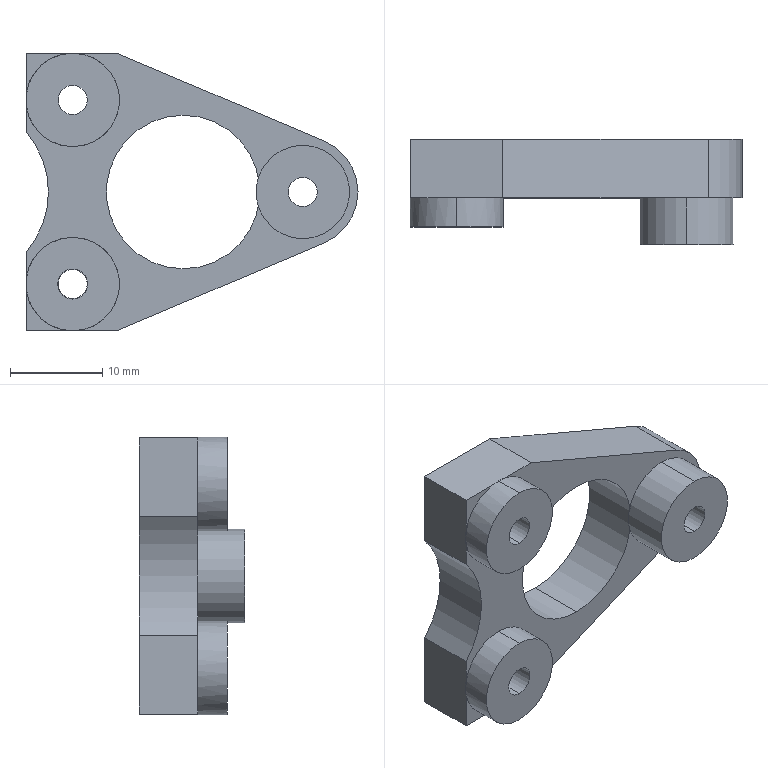Part | SolidWorks | features BaseBody 2 | 2 solids | 39 faces | box 36.08 x 11.43 x 30.16 mm | volume 4168 mm3 | cylinder 20 | plane 19 | commonest cylinder face diameters 3.175 x8 10.16 x6 3.258 x2 16.667 x2 12 x1 20 x1
STEP:
#1=CARTESIAN_POINT('',(-12.,-3.175,-8.371));
#2=VERTEX_POINT('',#1);
#3=CARTESIAN_POINT('',(-12.,-3.175,-11.629));
#4=VERTEX_POINT('',#3);
#5=CARTESIAN_POINT('',(-12.,-3.175,-10.));
#6=DIRECTION('',(0.,-1.,0.));
#7=DIRECTION('',(0.,0.,1.));
#8=AXIS2_PLACEMENT_3D('',#5,#6,#7);
#9=CIRCLE('',#8,1.629);
#10=EDGE_CURVE('',#2,#4,#9,.T.);
#11=ORIENTED_EDGE('',*,*,#10,.T.);
#12=CARTESIAN_POINT('',(-12.,0.,-11.629));
#13=VERTEX_POINT('',#12);
#14=CARTESIAN_POINT('',(-12.,-3.175,-11.629));
#15=DIRECTION('',(0.,1.,0.));
#16=VECTOR('',#15,1000.);
#17=LINE('',#14,#16);
#18=EDGE_CURVE('',#4,#13,#17,.T.);
#19=ORIENTED_EDGE('',*,*,#18,.T.);
#20=CARTESIAN_POINT('',(-12.,0.,-8.371));
#21=VERTEX_POINT('',#20);
#22=CARTESIAN_POINT('',(-12.,0.,-10.));
#23=DIRECTION('',(0.,1.,0.));
#24=DIRECTION('',(0.,0.,1.));
#25=AXIS2_PLACEMENT_3D('',#22,#23,#24);
#26=CIRCLE('',#25,1.629);
#27=EDGE_CURVE('',#13,#21,#26,.T.);
#28=ORIENTED_EDGE('',*,*,#27,.T.);
#29=CARTESIAN_POINT('',(-12.,-3.175,-8.371));
#30=DIRECTION('',(0.,1.,0.));
#31=VECTOR('',#30,1000.);
#32=LINE('',#29,#31);
#33=EDGE_CURVE('',#2,#21,#32,.T.);
#34=ORIENTED_EDGE('',*,*,#33,.F.);
#35=EDGE_LOOP('',(#11,#19,#28,#34));
#36=FACE_OUTER_BOUND('',#35,.T.);
#37=CARTESIAN_POINT('',(-12.,-3.175,-10.));
#38=DIRECTION('',(0.,1.,0.));
#39=DIRECTION('',(0.,0.,1.));
#40=AXIS2_PLACEMENT_3D('',#37,#38,#39);
#41=CYLINDRICAL_SURFACE('',#40,1.629);
#42=ADVANCED_FACE('',(#36),#41,.F.);
#43=CARTESIAN_POINT('',(-12.,6.35,-11.588));
#44=VERTEX_POINT('',#43);
#45=CARTESIAN_POINT('',(-12.,6.35,-8.412));
#46=VERTEX_POINT('',#45);
#47=CARTESIAN_POINT('',(-12.,6.35,-10.));
#48=DIRECTION('',(0.,1.,0.));
#49=DIRECTION('',(0.,0.,-1.));
#50=AXIS2_PLACEMENT_3D('',#47,#48,#49);
#51=CIRCLE('',#50,1.588);
#52=EDGE_CURVE('',#44,#46,#51,.T.);
#53=ORIENTED_EDGE('',*,*,#52,.T.);
#54=CARTESIAN_POINT('',(-12.,0.,-8.412));
#55=VERTEX_POINT('',#54);
#56=CARTESIAN_POINT('',(-12.,6.35,-8.412));
#57=DIRECTION('',(0.,-1.,0.));
#58=VECTOR('',#57,1000.);
#59=LINE('',#56,#58);
#60=EDGE_CURVE('',#46,#55,#59,.T.);
#61=ORIENTED_EDGE('',*,*,#60,.T.);
#62=CARTESIAN_POINT('',(-12.,0.,-11.588));
#63=VERTEX_POINT('',#62);
#64=CARTESIAN_POINT('',(-12.,0.,-10.));
#65=DIRECTION('',(0.,-1.,0.));
#66=DIRECTION('',(0.,0.,-1.));
#67=AXIS2_PLACEMENT_3D('',#64,#65,#66);
#68=CIRCLE('',#67,1.588);
#69=EDGE_CURVE('',#55,#63,#68,.T.);
#70=ORIENTED_EDGE('',*,*,#69,.T.);
#71=CARTESIAN_POINT('',(-12.,6.35,-11.588));
#72=DIRECTION('',(0.,-1.,0.));
#73=VECTOR('',#72,1000.);
#74=LINE('',#71,#73);
#75=EDGE_CURVE('',#44,#63,#74,.T.);
#76=ORIENTED_EDGE('',*,*,#75,.F.);
#77=EDGE_LOOP('',(#53,#61,#70,#76));
#78=FACE_OUTER_BOUND('',#77,.T.);
#79=CARTESIAN_POINT('',(-12.,6.35,-10.));
#80=DIRECTION('',(0.,-1.,0.));
#81=DIRECTION('',(0.,0.,-1.));
#82=AXIS2_PLACEMENT_3D('',#79,#80,#81);
#83=CYLINDRICAL_SURFACE('',#82,1.588);
#84=ADVANCED_FACE('',(#78),#83,.F.);
#85=CARTESIAN_POINT('',(-12.,-3.175,-15.08));
#86=VERTEX_POINT('',#85);
#87=CARTESIAN_POINT('',(-12.,-3.175,-4.92));
#88=VERTEX_POINT('',#87);
#89=CARTESIAN_POINT('',(-12.,-3.175,-10.));
#90=DIRECTION('',(0.,-1.,0.));
#91=DIRECTION('',(0.,0.,1.));
#92=AXIS2_PLACEMENT_3D('',#89,#90,#91);
#93=CIRCLE('',#92,5.08);
#94=EDGE_CURVE('',#86,#88,#93,.T.);
#95=ORIENTED_EDGE('',*,*,#94,.F.);
#96=CARTESIAN_POINT('',(-12.,0.,-15.08));
#97=VERTEX_POINT('',#96);
#98=CARTESIAN_POINT('',(-12.,-3.175,-15.08));
#99=DIRECTION('',(0.,1.,0.));
#100=VECTOR('',#99,1000.);
#101=LINE('',#98,#100);
#102=EDGE_CURVE('',#86,#97,#101,.T.);
#103=ORIENTED_EDGE('',*,*,#102,.T.);
#104=CARTESIAN_POINT('',(-11.102,0.,-15.));
#105=VERTEX_POINT('',#104);
#106=CARTESIAN_POINT('',(-12.,0.,-10.));
#107=DIRECTION('',(0.,-1.,0.));
#108=DIRECTION('',(0.,0.,1.));
#109=AXIS2_PLACEMENT_3D('',#106,#107,#108);
#110=CIRCLE('',#109,5.08);
#111=EDGE_CURVE('',#97,#105,#110,.T.);
#112=ORIENTED_EDGE('',*,*,#111,.T.);
#113=CARTESIAN_POINT('',(-12.,0.,-4.92));
#114=VERTEX_POINT('',#113);
#115=CARTESIAN_POINT('',(-12.,0.,-10.));
#116=DIRECTION('',(0.,1.,0.));
#117=DIRECTION('',(0.,0.,1.));
#118=AXIS2_PLACEMENT_3D('',#115,#116,#117);
#119=CIRCLE('',#118,5.08);
#120=EDGE_CURVE('',#114,#105,#119,.T.);
#121=ORIENTED_EDGE('',*,*,#120,.F.);
#122=CARTESIAN_POINT('',(-12.,-3.175,-4.92));
#123=DIRECTION('',(0.,1.,0.));
#124=VECTOR('',#123,1000.);
#125=LINE('',#122,#124);
#126=EDGE_CURVE('',#88,#114,#125,.T.);
#127=ORIENTED_EDGE('',*,*,#126,.F.);
#128=EDGE_LOOP('',(#95,#103,#112,#121,#127));
#129=FACE_OUTER_BOUND('',#128,.T.);
#130=CARTESIAN_POINT('',(-12.,-3.175,-10.));
#131=DIRECTION('',(0.,1.,0.));
#132=DIRECTION('',(0.,0.,1.));
#133=AXIS2_PLACEMENT_3D('',#130,#131,#132);
#134=CYLINDRICAL_SURFACE('',#133,5.08);
#135=ADVANCED_FACE('',(#129),#134,.T.);
#136=CARTESIAN_POINT('',(13.,6.35,1.587));
#137=VERTEX_POINT('',#136);
#138=CARTESIAN_POINT('',(13.,6.35,-1.587));
#139=VERTEX_POINT('',#138);
#140=CARTESIAN_POINT('',(13.,6.35,0.));
#141=DIRECTION('',(0.,-1.,0.));
#142=DIRECTION('',(0.,0.,-1.));
#143=AXIS2_PLACEMENT_3D('',#140,#141,#142);
#144=CIRCLE('',#143,1.587);
#145=EDGE_CURVE('',#137,#139,#144,.T.);
#146=ORIENTED_EDGE('',*,*,#145,.F.);
#147=CARTESIAN_POINT('',(13.,0.,1.587));
#148=VERTEX_POINT('',#147);
#149=CARTESIAN_POINT('',(13.,6.35,1.587));
#150=DIRECTION('',(0.,-1.,0.));
#151=VECTOR('',#150,1000.);
#152=LINE('',#149,#151);
#153=EDGE_CURVE('',#137,#148,#152,.T.);
#154=ORIENTED_EDGE('',*,*,#153,.T.);
#155=CARTESIAN_POINT('',(13.,0.,-1.587));
#156=VERTEX_POINT('',#155);
#157=CARTESIAN_POINT('',(13.,0.,0.));
#158=DIRECTION('',(0.,-1.,0.));
#159=DIRECTION('',(0.,0.,-1.));
#160=AXIS2_PLACEMENT_3D('',#157,#158,#159);
#161=CIRCLE('',#160,1.587);
#162=EDGE_CURVE('',#148,#156,#161,.T.);
#163=ORIENTED_EDGE('',*,*,#162,.T.);
#164=CARTESIAN_POINT('',(13.,6.35,-1.587));
#165=DIRECTION('',(0.,-1.,0.));
#166=VECTOR('',#165,1000.);
#167=LINE('',#164,#166);
#168=EDGE_CURVE('',#139,#156,#167,.T.);
#169=ORIENTED_EDGE('',*,*,#168,.F.);
#170=EDGE_LOOP('',(#146,#154,#163,#169));
#171=FACE_OUTER_BOUND('',#170,.T.);
#172=CARTESIAN_POINT('',(13.,6.35,0.));
#173=DIRECTION('',(0.,-1.,0.));
#174=DIRECTION('',(0.,0.,-1.));
#175=AXIS2_PLACEMENT_3D('',#172,#173,#174);
#176=CYLINDRICAL_SURFACE('',#175,1.587);
#177=ADVANCED_FACE('',(#171),#176,.F.);
#178=CARTESIAN_POINT('',(-12.,6.35,11.587));
#179=VERTEX_POINT('',#178);
#180=CARTESIAN_POINT('',(-12.,6.35,8.413));
#181=VERTEX_POINT('',#180);
#182=CARTESIAN_POINT('',(-12.,6.35,10.));
#183=DIRECTION('',(0.,-1.,0.));
#184=DIRECTION('',(0.,0.,-1.));
#185=AXIS2_PLACEMENT_3D('',#182,#183,#184);
#186=CIRCLE('',#185,1.587);
#187=EDGE_CURVE('',#179,#181,#186,.T.);
#188=ORIENTED_EDGE('',*,*,#187,.F.);
#189=CARTESIAN_POINT('',(-12.,-3.175,11.587));
#190=VERTEX_POINT('',#189);
#191=CARTESIAN_POINT('',(-12.,6.35,11.587));
#192=DIRECTION('',(0.,-1.,0.));
#193=VECTOR('',#192,1000.);
#194=LINE('',#191,#193);
#195=EDGE_CURVE('',#179,#190,#194,.T.);
#196=ORIENTED_EDGE('',*,*,#195,.T.);
#197=CARTESIAN_POINT('',(-12.,-3.175,8.413));
#198=VERTEX_POINT('',#197);
#199=CARTESIAN_POINT('',(-12.,-3.175,10.));
#200=DIRECTION('',(0.,-1.,0.));
#201=DIRECTION('',(0.,0.,-1.));
#202=AXIS2_PLACEMENT_3D('',#199,#200,#201);
#203=CIRCLE('',#202,1.587);
#204=EDGE_CURVE('',#190,#198,#203,.T.);
#205=ORIENTED_EDGE('',*,*,#204,.T.);
#206=CARTESIAN_POINT('',(-12.,6.35,8.413));
#207=DIRECTION('',(0.,-1.,0.));
#208=VECTOR('',#207,1000.);
#209=LINE('',#206,#208);
#210=EDGE_CURVE('',#181,#198,#209,.T.);
#211=ORIENTED_EDGE('',*,*,#210,.F.);
#212=EDGE_LOOP('',(#188,#196,#205,#211));
#213=FACE_OUTER_BOUND('',#212,.T.);
#214=CARTESIAN_POINT('',(-12.,6.35,10.));
#215=DIRECTION('',(0.,-1.,0.));
#216=DIRECTION('',(0.,0.,-1.));
#217=AXIS2_PLACEMENT_3D('',#214,#215,#216);
#218=CYLINDRICAL_SURFACE('',#217,1.587);
#219=ADVANCED_FACE('',(#213),#218,.F.);
#220=CARTESIAN_POINT('',(0.,6.35,8.334));
#221=VERTEX_POINT('',#220);
#222=CARTESIAN_POINT('',(0.,6.35,-8.334));
#223=VERTEX_POINT('',#222);
#224=CARTESIAN_POINT('',(0.,6.35,0.));
#225=DIRECTION('',(0.,-1.,0.));
#226=DIRECTION('',(0.,0.,-1.));
#227=AXIS2_PLACEMENT_3D('',#224,#225,#226);
#228=CIRCLE('',#227,8.334);
#229=EDGE_CURVE('',#221,#223,#228,.T.);
#230=ORIENTED_EDGE('',*,*,#229,.F.);
#231=CARTESIAN_POINT('',(0.,0.,8.334));
#232=VERTEX_POINT('',#231);
#233=CARTESIAN_POINT('',(0.,6.35,8.334));
#234=DIRECTION('',(0.,-1.,0.));
#235=VECTOR('',#234,1000.);
#236=LINE('',#233,#235);
#237=EDGE_CURVE('',#221,#232,#236,.T.);
#238=ORIENTED_EDGE('',*,*,#237,.T.);
#239=CARTESIAN_POINT('',(0.,0.,-8.334));
#240=VERTEX_POINT('',#239);
#241=CARTESIAN_POINT('',(0.,0.,0.));
#242=DIRECTION('',(0.,-1.,0.));
#243=DIRECTION('',(0.,0.,-1.));
#244=AXIS2_PLACEMENT_3D('',#241,#242,#243);
#245=CIRCLE('',#244,8.334);
#246=EDGE_CURVE('',#232,#240,#245,.T.);
#247=ORIENTED_EDGE('',*,*,#246,.T.);
#248=CARTESIAN_POINT('',(0.,6.35,-8.334));
#249=DIRECTION('',(0.,-1.,0.));
#250=VECTOR('',#249,1000.);
#251=LINE('',#248,#250);
#252=EDGE_CURVE('',#223,#240,#251,.T.);
#253=ORIENTED_EDGE('',*,*,#252,.F.);
#254=EDGE_LOOP('',(#230,#238,#247,#253));
#255=FACE_OUTER_BOUND('',#254,.T.);
#256=CARTESIAN_POINT('',(0.,6.35,0.));
#257=DIRECTION('',(0.,-1.,0.));
#258=DIRECTION('',(0.,0.,-1.));
#259=AXIS2_PLACEMENT_3D('',#256,#257,#258);
#260=CYLINDRICAL_SURFACE('',#259,8.334);
#261=ADVANCED_FACE('',(#255),#260,.F.);
#262=CARTESIAN_POINT('',(-12.,-3.175,4.92));
#263=VERTEX_POINT('',#262);
#264=CARTESIAN_POINT('',(-12.,-3.175,15.08));
#265=VERTEX_POINT('',#264);
#266=CARTESIAN_POINT('',(-12.,-3.175,10.));
#267=DIRECTION('',(0.,-1.,0.));
#268=DIRECTION('',(0.,0.,1.));
#269=AXIS2_PLACEMENT_3D('',#266,#267,#268);
#270=CIRCLE('',#269,5.08);
#271=EDGE_CURVE('',#263,#265,#270,.T.);
#272=ORIENTED_EDGE('',*,*,#271,.F.);
#273=CARTESIAN_POINT('',(-12.,0.,4.92));
#274=VERTEX_POINT('',#273);
#275=CARTESIAN_POINT('',(-12.,-3.175,4.92));
#276=DIRECTION('',(0.,1.,0.));
#277=VECTOR('',#276,1000.);
#278=LINE('',#275,#277);
#279=EDGE_CURVE('',#263,#274,#278,.T.);
#280=ORIENTED_EDGE('',*,*,#279,.T.);
#281=CARTESIAN_POINT('',(-11.102,0.,15.));
#282=VERTEX_POINT('',#281);
#283=CARTESIAN_POINT('',(-12.,0.,10.));
#284=DIRECTION('',(0.,-1.,0.));
#285=DIRECTION('',(0.,0.,1.));
#286=AXIS2_PLACEMENT_3D('',#283,#284,#285);
#287=CIRCLE('',#286,5.08);
#288=EDGE_CURVE('',#274,#282,#287,.T.);
#289=ORIENTED_EDGE('',*,*,#288,.T.);
#290=CARTESIAN_POINT('',(-12.,0.,15.08));
#291=VERTEX_POINT('',#290);
#292=CARTESIAN_POINT('',(-12.,0.,10.));
#293=DIRECTION('',(0.,1.,0.));
#294=DIRECTION('',(0.,0.,1.));
#295=AXIS2_PLACEMENT_3D('',#292,#293,#294);
#296=CIRCLE('',#295,5.08);
#297=EDGE_CURVE('',#291,#282,#296,.T.);
#298=ORIENTED_EDGE('',*,*,#297,.F.);
#299=CARTESIAN_POINT('',(-12.,-3.175,15.08));
#300=DIRECTION('',(0.,1.,0.));
#301=VECTOR('',#300,1000.);
#302=LINE('',#299,#301);
#303=EDGE_CURVE('',#265,#291,#302,.T.);
#304=ORIENTED_EDGE('',*,*,#303,.F.);
#305=EDGE_LOOP('',(#272,#280,#289,#298,#304));
#306=FACE_OUTER_BOUND('',#305,.T.);
#307=CARTESIAN_POINT('',(-12.,-3.175,10.));
#308=DIRECTION('',(0.,1.,0.));
#309=DIRECTION('',(0.,0.,1.));
#310=AXIS2_PLACEMENT_3D('',#307,#308,#309);
#311=CYLINDRICAL_SURFACE('',#310,5.08);
#312=ADVANCED_FACE('',(#306),#311,.T.);
#313=ORIENTED_EDGE('',*,*,#18,.F.);
#314=CARTESIAN_POINT('',(-12.,-3.175,-10.));
#315=DIRECTION('',(0.,-1.,0.));
#316=DIRECTION('',(0.,0.,1.));
#317=AXIS2_PLACEMENT_3D('',#314,#315,#316);
#318=CIRCLE('',#317,1.629);
#319=EDGE_CURVE('',#4,#2,#318,.T.);
#320=ORIENTED_EDGE('',*,*,#319,.T.);
#321=ORIENTED_EDGE('',*,*,#33,.T.);
#322=CARTESIAN_POINT('',(-12.,0.,-10.));
#323=DIRECTION('',(0.,1.,0.));
#324=DIRECTION('',(0.,0.,1.));
#325=AXIS2_PLACEMENT_3D('',#322,#323,#324);
#326=CIRCLE('',#325,1.629);
#327=EDGE_CURVE('',#21,#13,#326,.T.);
#328=ORIENTED_EDGE('',*,*,#327,.T.);
#329=EDGE_LOOP('',(#313,#320,#321,#328));
#330=FACE_OUTER_BOUND('',#329,.T.);
#331=CARTESIAN_POINT('',(-12.,-3.175,-10.));
#332=DIRECTION('',(0.,1.,0.));
#333=DIRECTION('',(0.,0.,1.));
#334=AXIS2_PLACEMENT_3D('',#331,#332,#333);
#335=CYLINDRICAL_SURFACE('',#334,1.629);
#336=ADVANCED_FACE('',(#330),#335,.F.);
#337=CARTESIAN_POINT('',(-12.,0.,-10.));
#338=DIRECTION('',(0.,-1.,0.));
#339=DIRECTION('',(0.,0.,-1.));
#340=AXIS2_PLACEMENT_3D('',#337,#338,#339);
#341=CIRCLE('',#340,1.588);
#342=EDGE_CURVE('',#63,#55,#341,.T.);
#343=ORIENTED_EDGE('',*,*,#342,.F.);
#344=ORIENTED_EDGE('',*,*,#69,.F.);
#345=EDGE_LOOP('',(#343,#344));
#346=FACE_BOUND('',#345,.T.);
#347=ORIENTED_EDGE('',*,*,#327,.F.);
#348=ORIENTED_EDGE('',*,*,#27,.F.);
#349=EDGE_LOOP('',(#347,#348));
#350=FACE_OUTER_BOUND('',#349,.T.);
#351=CARTESIAN_POINT('',(-13.649,0.,-11.649));
#352=DIRECTION('',(0.,1.,0.));
#353=DIRECTION('',(0.,0.,1.));
#354=AXIS2_PLACEMENT_3D('',#351,#352,#353);
#355=PLANE('',#354);
#356=ADVANCED_FACE('',(#346,#350),#355,.F.);
#357=ORIENTED_EDGE('',*,*,#10,.F.);
#358=ORIENTED_EDGE('',*,*,#319,.F.);
#359=EDGE_LOOP('',(#357,#358));
#360=FACE_BOUND('',#359,.T.);
#361=CARTESIAN_POINT('',(-12.,-3.175,-10.));
#362=DIRECTION('',(0.,-1.,0.));
#363=DIRECTION('',(0.,0.,1.));
#364=AXIS2_PLACEMENT_3D('',#361,#362,#363);
#365=CIRCLE('',#364,5.08);
#366=EDGE_CURVE('',#88,#86,#365,.T.);
#367=ORIENTED_EDGE('',*,*,#366,.T.);
#368=ORIENTED_EDGE('',*,*,#94,.T.);
#369=EDGE_LOOP('',(#367,#368));
#370=FACE_OUTER_BOUND('',#369,.T.);
#371=CARTESIAN_POINT('',(-17.141,-3.175,-4.859));
#372=DIRECTION('',(0.,-1.,0.));
#373=DIRECTION('',(0.,0.,-1.));
#374=AXIS2_PLACEMENT_3D('',#371,#372,#373);
#375=PLANE('',#374);
#376=ADVANCED_FACE('',(#360,#370),#375,.T.);
#377=ORIENTED_EDGE('',*,*,#60,.F.);
#378=CARTESIAN_POINT('',(-12.,6.35,-10.));
#379=DIRECTION('',(0.,1.,0.));
#380=DIRECTION('',(0.,0.,-1.));
#381=AXIS2_PLACEMENT_3D('',#378,#379,#380);
#382=CIRCLE('',#381,1.588);
#383=EDGE_CURVE('',#46,#44,#382,.T.);
#384=ORIENTED_EDGE('',*,*,#383,.T.);
#385=ORIENTED_EDGE('',*,*,#75,.T.);
#386=ORIENTED_EDGE('',*,*,#342,.T.);
#387=EDGE_LOOP('',(#377,#384,#385,#386));
#388=FACE_OUTER_BOUND('',#387,.T.);
#389=CARTESIAN_POINT('',(-12.,6.35,-10.));
#390=DIRECTION('',(0.,-1.,0.));
#391=DIRECTION('',(0.,0.,-1.));
#392=AXIS2_PLACEMENT_3D('',#389,#390,#391);
#393=CYLINDRICAL_SURFACE('',#392,1.588);
#394=ADVANCED_FACE('',(#388),#393,.F.);
#395=ORIENTED_EDGE('',*,*,#102,.F.);
#396=ORIENTED_EDGE('',*,*,#366,.F.);
#397=ORIENTED_EDGE('',*,*,#126,.T.);
#398=CARTESIAN_POINT('',(-17.,0.,-9.102));
#399=VERTEX_POINT('',#398);
#400=CARTESIAN_POINT('',(-12.,0.,-10.));
#401=DIRECTION('',(0.,1.,0.));
#402=DIRECTION('',(0.,0.,1.));
#403=AXIS2_PLACEMENT_3D('',#400,#401,#402);
#404=CIRCLE('',#403,5.08);
#405=EDGE_CURVE('',#399,#114,#404,.T.);
#406=ORIENTED_EDGE('',*,*,#405,.F.);
#407=CARTESIAN_POINT('',(-17.,0.,-10.898));
#408=VERTEX_POINT('',#407);
#409=CARTESIAN_POINT('',(-12.,0.,-10.));
#410=DIRECTION('',(0.,1.,0.));
#411=DIRECTION('',(0.,0.,1.));
#412=AXIS2_PLACEMENT_3D('',#409,#410,#411);
#413=CIRCLE('',#412,5.08);
#414=EDGE_CURVE('',#408,#399,#413,.T.);
#415=ORIENTED_EDGE('',*,*,#414,.F.);
#416=CARTESIAN_POINT('',(-12.898,0.,-15.));
#417=VERTEX_POINT('',#416);
#418=CARTESIAN_POINT('',(-12.,0.,-10.));
#419=DIRECTION('',(0.,1.,0.));
#420=DIRECTION('',(0.,0.,1.));
#421=AXIS2_PLACEMENT_3D('',#418,#419,#420);
#422=CIRCLE('',#421,5.08);
#423=EDGE_CURVE('',#417,#408,#422,.T.);
#424=ORIENTED_EDGE('',*,*,#423,.F.);
#425=CARTESIAN_POINT('',(-12.,0.,-10.));
#426=DIRECTION('',(0.,-1.,0.));
#427=DIRECTION('',(0.,0.,1.));
#428=AXIS2_PLACEMENT_3D('',#425,#426,#427);
#429=CIRCLE('',#428,5.08);
#430=EDGE_CURVE('',#417,#97,#429,.T.);
#431=ORIENTED_EDGE('',*,*,#430,.T.);
#432=EDGE_LOOP('',(#395,#396,#397,#406,#415,#424,#431));
#433=FACE_OUTER_BOUND('',#432,.T.);
#434=CARTESIAN_POINT('',(-12.,-3.175,-10.));
#435=DIRECTION('',(0.,1.,0.));
#436=DIRECTION('',(0.,0.,1.));
#437=AXIS2_PLACEMENT_3D('',#434,#435,#436);
#438=CYLINDRICAL_SURFACE('',#437,5.08);
#439=ADVANCED_FACE('',(#433),#438,.T.);
#440=CARTESIAN_POINT('',(13.,6.35,0.));
#441=DIRECTION('',(0.,-1.,0.));
#442=DIRECTION('',(0.,0.,-1.));
#443=AXIS2_PLACEMENT_3D('',#440,#441,#442);
#444=CIRCLE('',#443,1.587);
#445=EDGE_CURVE('',#139,#137,#444,.T.);
#446=ORIENTED_EDGE('',*,*,#445,.T.);
#447=ORIENTED_EDGE('',*,*,#145,.T.);
#448=EDGE_LOOP('',(#446,#447));
#449=FACE_BOUND('',#448,.T.);
#450=CARTESIAN_POINT('',(-12.,6.35,10.));
#451=DIRECTION('',(0.,-1.,0.));
#452=DIRECTION('',(0.,0.,-1.));
#453=AXIS2_PLACEMENT_3D('',#450,#451,#452);
#454=CIRCLE('',#453,1.587);
#455=EDGE_CURVE('',#181,#179,#454,.T.);
#456=ORIENTED_EDGE('',*,*,#455,.T.);
#457=ORIENTED_EDGE('',*,*,#187,.T.);
#458=EDGE_LOOP('',(#456,#457));
#459=FACE_BOUND('',#458,.T.);
#460=ORIENTED_EDGE('',*,*,#52,.F.);
#461=ORIENTED_EDGE('',*,*,#383,.F.);
#462=EDGE_LOOP('',(#460,#461));
#463=FACE_BOUND('',#462,.T.);
#464=CARTESIAN_POINT('',(0.,6.35,0.));
#465=DIRECTION('',(0.,-1.,0.));
#466=DIRECTION('',(0.,0.,-1.));
#467=AXIS2_PLACEMENT_3D('',#464,#465,#466);
#468=CIRCLE('',#467,8.334);
#469=EDGE_CURVE('',#223,#221,#468,.T.);
#470=ORIENTED_EDGE('',*,*,#469,.T.);
#471=ORIENTED_EDGE('',*,*,#229,.T.);
#472=EDGE_LOOP('',(#470,#471));
#473=FACE_BOUND('',#472,.T.);
#474=CARTESIAN_POINT('',(-17.,6.35,-6.455));
#475=VERTEX_POINT('',#474);
#476=CARTESIAN_POINT('',(-17.,6.35,6.455));
#477=VERTEX_POINT('',#476);
#478=CARTESIAN_POINT('',(-24.638,6.35,0.));
#479=DIRECTION('',(0.,-1.,0.));
#480=DIRECTION('',(0.,0.,-1.));
#481=AXIS2_PLACEMENT_3D('',#478,#479,#480);
#482=CIRCLE('',#481,10.);
#483=EDGE_CURVE('',#475,#477,#482,.T.);
#484=ORIENTED_EDGE('',*,*,#483,.T.);
#485=CARTESIAN_POINT('',(-17.,6.35,15.));
#486=VERTEX_POINT('',#485);
#487=CARTESIAN_POINT('',(-17.,6.35,0.));
#488=DIRECTION('',(0.,0.,1.));
#489=VECTOR('',#488,1000.);
#490=LINE('',#487,#489);
#491=EDGE_CURVE('',#477,#486,#490,.T.);
#492=ORIENTED_EDGE('',*,*,#491,.T.);
#493=CARTESIAN_POINT('',(-7.,6.35,15.));
#494=VERTEX_POINT('',#493);
#495=CARTESIAN_POINT('',(1.108,6.35,15.));
#496=DIRECTION('',(1.,0.,0.));
#497=VECTOR('',#496,1000.);
#498=LINE('',#495,#497);
#499=EDGE_CURVE('',#486,#494,#498,.T.);
#500=ORIENTED_EDGE('',*,*,#499,.T.);
#501=CARTESIAN_POINT('',(15.343,6.35,5.524));
#502=VERTEX_POINT('',#501);
#503=CARTESIAN_POINT('',(-7.,6.35,15.));
#504=DIRECTION('',(0.9206,0.,-0.3905));
#505=VECTOR('',#504,1000.);
#506=LINE('',#503,#505);
#507=EDGE_CURVE('',#494,#502,#506,.T.);
#508=ORIENTED_EDGE('',*,*,#507,.T.);
#509=CARTESIAN_POINT('',(15.343,6.35,-5.524));
#510=VERTEX_POINT('',#509);
#511=CARTESIAN_POINT('',(13.,6.35,0.));
#512=DIRECTION('',(0.,1.,0.));
#513=DIRECTION('',(0.,0.,-1.));
#514=AXIS2_PLACEMENT_3D('',#511,#512,#513);
#515=CIRCLE('',#514,6.);
#516=EDGE_CURVE('',#502,#510,#515,.T.);
#517=ORIENTED_EDGE('',*,*,#516,.T.);
#518=CARTESIAN_POINT('',(-7.,6.35,-15.));
#519=VERTEX_POINT('',#518);
#520=CARTESIAN_POINT('',(15.343,6.35,-5.524));
#521=DIRECTION('',(-0.9206,0.,-0.3905));
#522=VECTOR('',#521,1000.);
#523=LINE('',#520,#522);
#524=EDGE_CURVE('',#510,#519,#523,.T.);
#525=ORIENTED_EDGE('',*,*,#524,.T.);
#526=CARTESIAN_POINT('',(-17.,6.35,-15.));
#527=VERTEX_POINT('',#526);
#528=CARTESIAN_POINT('',(1.108,6.35,-15.));
#529=DIRECTION('',(-1.,0.,0.));
#530=VECTOR('',#529,1000.);
#531=LINE('',#528,#530);
#532=EDGE_CURVE('',#519,#527,#531,.T.);
#533=ORIENTED_EDGE('',*,*,#532,.T.);
#534=CARTESIAN_POINT('',(-17.,6.35,0.));
#535=DIRECTION('',(0.,0.,1.));
#536=VECTOR('',#535,1000.);
#537=LINE('',#534,#536);
#538=EDGE_CURVE('',#527,#475,#537,.T.);
#539=ORIENTED_EDGE('',*,*,#538,.T.);
#540=EDGE_LOOP('',(#484,#492,#500,#508,#517,#525,#533,#539));
#541=FACE_OUTER_BOUND('',#540,.T.);
#542=CARTESIAN_POINT('',(-17.,6.35,-15.));
#543=DIRECTION('',(0.,1.,0.));
#544=DIRECTION('',(0.,0.,1.));
#545=AXIS2_PLACEMENT_3D('',#542,#543,#544);
#546=PLANE('',#545);
#547=ADVANCED_FACE('',(#449,#459,#463,#473,#541),#546,.T.);
#548=CARTESIAN_POINT('',(0.,0.,0.));
#549=DIRECTION('',(0.,-1.,0.));
#550=DIRECTION('',(0.,0.,-1.));
#551=AXIS2_PLACEMENT_3D('',#548,#549,#550);
#552=CIRCLE('',#551,8.334);
#553=EDGE_CURVE('',#240,#232,#552,.T.);
#554=ORIENTED_EDGE('',*,*,#553,.F.);
#555=ORIENTED_EDGE('',*,*,#246,.F.);
#556=EDGE_LOOP('',(#554,#555));
#557=FACE_BOUND('',#556,.T.);
#558=CARTESIAN_POINT('',(13.,0.,0.));
#559=DIRECTION('',(0.,-1.,0.));
#560=DIRECTION('',(0.,0.,-1.));
#561=AXIS2_PLACEMENT_3D('',#558,#559,#560);
#562=CIRCLE('',#561,1.587);
#563=EDGE_CURVE('',#156,#148,#562,.T.);
#564=ORIENTED_EDGE('',*,*,#563,.F.);
#565=ORIENTED_EDGE('',*,*,#162,.F.);
#566=EDGE_LOOP('',(#564,#565));
#567=FACE_BOUND('',#566,.T.);
#568=CARTESIAN_POINT('',(-7.,0.,-15.));
#569=VERTEX_POINT('',#568);
#570=CARTESIAN_POINT('',(1.108,0.,-15.));
#571=DIRECTION('',(-1.,0.,0.));
#572=VECTOR('',#571,1000.);
#573=LINE('',#570,#572);
#574=EDGE_CURVE('',#569,#105,#573,.T.);
#575=ORIENTED_EDGE('',*,*,#574,.F.);
#576=CARTESIAN_POINT('',(15.343,0.,-5.524));
#577=VERTEX_POINT('',#576);
#578=CARTESIAN_POINT('',(-7.,0.,-15.));
#579=DIRECTION('',(-0.9206,0.,-0.3905));
#580=VECTOR('',#579,1000.);
#581=LINE('',#578,#580);
#582=EDGE_CURVE('',#577,#569,#581,.T.);
#583=ORIENTED_EDGE('',*,*,#582,.F.);
#584=CARTESIAN_POINT('',(15.343,0.,5.524));
#585=VERTEX_POINT('',#584);
#586=CARTESIAN_POINT('',(13.,0.,0.));
#587=DIRECTION('',(0.,1.,0.));
#588=DIRECTION('',(0.,0.,-1.));
#589=AXIS2_PLACEMENT_3D('',#586,#587,#588);
#590=CIRCLE('',#589,6.);
#591=EDGE_CURVE('',#585,#577,#590,.T.);
#592=ORIENTED_EDGE('',*,*,#591,.F.);
#593=CARTESIAN_POINT('',(-7.,0.,15.));
#594=VERTEX_POINT('',#593);
#595=CARTESIAN_POINT('',(15.343,0.,5.524));
#596=DIRECTION('',(0.9206,0.,-0.3905));
#597=VECTOR('',#596,1000.);
#598=LINE('',#595,#597);
#599=EDGE_CURVE('',#594,#585,#598,.T.);
#600=ORIENTED_EDGE('',*,*,#599,.F.);
#601=CARTESIAN_POINT('',(1.108,0.,15.));
#602=DIRECTION('',(1.,0.,0.));
#603=VECTOR('',#602,1000.);
#604=LINE('',#601,#603);
#605=EDGE_CURVE('',#282,#594,#604,.T.);
#606=ORIENTED_EDGE('',*,*,#605,.F.);
#607=ORIENTED_EDGE('',*,*,#288,.F.);
#608=CARTESIAN_POINT('',(-17.,0.,9.102));
#609=VERTEX_POINT('',#608);
#610=CARTESIAN_POINT('',(-12.,0.,10.));
#611=DIRECTION('',(0.,-1.,0.));
#612=DIRECTION('',(0.,0.,1.));
#613=AXIS2_PLACEMENT_3D('',#610,#611,#612);
#614=CIRCLE('',#613,5.08);
#615=EDGE_CURVE('',#609,#274,#614,.T.);
#616=ORIENTED_EDGE('',*,*,#615,.F.);
#617=CARTESIAN_POINT('',(-17.,0.,6.455));
#618=VERTEX_POINT('',#617);
#619=CARTESIAN_POINT('',(-17.,0.,0.));
#620=DIRECTION('',(0.,0.,1.));
#621=VECTOR('',#620,1000.);
#622=LINE('',#619,#621);
#623=EDGE_CURVE('',#618,#609,#622,.T.);
#624=ORIENTED_EDGE('',*,*,#623,.F.);
#625=CARTESIAN_POINT('',(-17.,0.,-6.455));
#626=VERTEX_POINT('',#625);
#627=CARTESIAN_POINT('',(-24.638,0.,0.));
#628=DIRECTION('',(0.,-1.,0.));
#629=DIRECTION('',(0.,0.,-1.));
#630=AXIS2_PLACEMENT_3D('',#627,#628,#629);
#631=CIRCLE('',#630,10.);
#632=EDGE_CURVE('',#626,#618,#631,.T.);
#633=ORIENTED_EDGE('',*,*,#632,.F.);
#634=CARTESIAN_POINT('',(-17.,0.,0.));
#635=DIRECTION('',(0.,0.,1.));
#636=VECTOR('',#635,1000.);
#637=LINE('',#634,#636);
#638=EDGE_CURVE('',#399,#626,#637,.T.);
#639=ORIENTED_EDGE('',*,*,#638,.F.);
#640=ORIENTED_EDGE('',*,*,#405,.T.);
#641=ORIENTED_EDGE('',*,*,#120,.T.);
#642=EDGE_LOOP('',(#575,#583,#592,#600,#606,#607,#616,#624,#633,#639,#640,#641));
#643=FACE_OUTER_BOUND('',#642,.T.);
#644=CARTESIAN_POINT('',(-17.,0.,-15.));
#645=DIRECTION('',(0.,1.,0.));
#646=DIRECTION('',(0.,0.,1.));
#647=AXIS2_PLACEMENT_3D('',#644,#645,#646);
#648=PLANE('',#647);
#649=ADVANCED_FACE('',(#557,#567,#643),#648,.F.);
#650=CARTESIAN_POINT('',(-17.,0.,-10.));
#651=DIRECTION('',(0.,0.,1.));
#652=VECTOR('',#651,1000.);
#653=LINE('',#650,#652);
#654=EDGE_CURVE('',#408,#399,#653,.T.);
#655=ORIENTED_EDGE('',*,*,#654,.F.);
#656=ORIENTED_EDGE('',*,*,#414,.T.);
#657=EDGE_LOOP('',(#655,#656));
#658=FACE_OUTER_BOUND('',#657,.T.);
#659=CARTESIAN_POINT('',(-17.08,0.,-9.091));
#660=DIRECTION('',(0.,-1.,0.));
#661=DIRECTION('',(0.,0.,-1.));
#662=AXIS2_PLACEMENT_3D('',#659,#660,#661);
#663=PLANE('',#662);
#664=ADVANCED_FACE('',(#658),#663,.F.);
#665=CARTESIAN_POINT('',(-17.,0.,-15.));
#666=VERTEX_POINT('',#665);
#667=CARTESIAN_POINT('',(-17.,0.,-12.937));
#668=DIRECTION('',(0.,0.,1.));
#669=VECTOR('',#668,1000.);
#670=LINE('',#667,#669);
#671=EDGE_CURVE('',#666,#408,#670,.T.);
#672=ORIENTED_EDGE('',*,*,#671,.F.);
#673=CARTESIAN_POINT('',(-14.937,0.,-15.));
#674=DIRECTION('',(-1.,0.,0.));
#675=VECTOR('',#674,1000.);
#676=LINE('',#673,#675);
#677=EDGE_CURVE('',#417,#666,#676,.T.);
#678=ORIENTED_EDGE('',*,*,#677,.F.);
#679=ORIENTED_EDGE('',*,*,#423,.T.);
#680=EDGE_LOOP('',(#672,#678,#679));
#681=FACE_OUTER_BOUND('',#680,.T.);
#682=CARTESIAN_POINT('',(-17.,0.,-15.));
#683=DIRECTION('',(0.,1.,0.));
#684=DIRECTION('',(0.,0.,1.));
#685=AXIS2_PLACEMENT_3D('',#682,#683,#684);
#686=PLANE('',#685);
#687=ADVANCED_FACE('',(#681),#686,.F.);
#688=ORIENTED_EDGE('',*,*,#153,.F.);
#689=ORIENTED_EDGE('',*,*,#445,.F.);
#690=ORIENTED_EDGE('',*,*,#168,.T.);
#691=ORIENTED_EDGE('',*,*,#563,.T.);
#692=EDGE_LOOP('',(#688,#689,#690,#691));
#693=FACE_OUTER_BOUND('',#692,.T.);
#694=CARTESIAN_POINT('',(13.,6.35,0.));
#695=DIRECTION('',(0.,-1.,0.));
#696=DIRECTION('',(0.,0.,-1.));
#697=AXIS2_PLACEMENT_3D('',#694,#695,#696);
#698=CYLINDRICAL_SURFACE('',#697,1.587);
#699=ADVANCED_FACE('',(#693),#698,.F.);
#700=ORIENTED_EDGE('',*,*,#195,.F.);
#701=ORIENTED_EDGE('',*,*,#455,.F.);
#702=ORIENTED_EDGE('',*,*,#210,.T.);
#703=CARTESIAN_POINT('',(-12.,-3.175,10.));
#704=DIRECTION('',(0.,-1.,0.));
#705=DIRECTION('',(0.,0.,-1.));
#706=AXIS2_PLACEMENT_3D('',#703,#704,#705);
#707=CIRCLE('',#706,1.587);
#708=EDGE_CURVE('',#198,#190,#707,.T.);
#709=ORIENTED_EDGE('',*,*,#708,.T.);
#710=EDGE_LOOP('',(#700,#701,#702,#709));
#711=FACE_OUTER_BOUND('',#710,.T.);
#712=CARTESIAN_POINT('',(-12.,6.35,10.));
#713=DIRECTION('',(0.,-1.,0.));
#714=DIRECTION('',(0.,0.,-1.));
#715=AXIS2_PLACEMENT_3D('',#712,#713,#714);
#716=CYLINDRICAL_SURFACE('',#715,1.587);
#717=ADVANCED_FACE('',(#711),#716,.F.);
#718=ORIENTED_EDGE('',*,*,#237,.F.);
#719=ORIENTED_EDGE('',*,*,#469,.F.);
#720=ORIENTED_EDGE('',*,*,#252,.T.);
#721=ORIENTED_EDGE('',*,*,#553,.T.);
#722=EDGE_LOOP('',(#718,#719,#720,#721));
#723=FACE_OUTER_BOUND('',#722,.T.);
#724=CARTESIAN_POINT('',(0.,6.35,0.));
#725=DIRECTION('',(0.,-1.,0.));
#726=DIRECTION('',(0.,0.,-1.));
#727=AXIS2_PLACEMENT_3D('',#724,#725,#726);
#728=CYLINDRICAL_SURFACE('',#727,8.334);
#729=ADVANCED_FACE('',(#723),#728,.F.);
#730=CARTESIAN_POINT('',(-17.,0.,10.898));
#731=VERTEX_POINT('',#730);
#732=CARTESIAN_POINT('',(-17.,0.,10.727));
#733=DIRECTION('',(0.,0.,-1.));
#734=VECTOR('',#733,1000.);
#735=LINE('',#732,#734);
#736=EDGE_CURVE('',#731,#609,#735,.T.);
#737=ORIENTED_EDGE('',*,*,#736,.F.);
#738=CARTESIAN_POINT('',(-17.,0.,15.));
#739=VERTEX_POINT('',#738);
#740=CARTESIAN_POINT('',(-17.,0.,10.727));
#741=DIRECTION('',(0.,0.,-1.));
#742=VECTOR('',#741,1000.);
#743=LINE('',#740,#742);
#744=EDGE_CURVE('',#739,#731,#743,.T.);
#745=ORIENTED_EDGE('',*,*,#744,.F.);
#746=CARTESIAN_POINT('',(-17.,3.175,15.));
#747=DIRECTION('',(0.,-1.,0.));
#748=VECTOR('',#747,1000.);
#749=LINE('',#746,#748);
#750=EDGE_CURVE('',#486,#739,#749,.T.);
#751=ORIENTED_EDGE('',*,*,#750,.F.);
#752=ORIENTED_EDGE('',*,*,#491,.F.);
#753=CARTESIAN_POINT('',(-17.,3.175,6.455));
#754=DIRECTION('',(0.,1.,0.));
#755=VECTOR('',#754,1000.);
#756=LINE('',#753,#755);
#757=EDGE_CURVE('',#618,#477,#756,.T.);
#758=ORIENTED_EDGE('',*,*,#757,.F.);
#759=ORIENTED_EDGE('',*,*,#623,.T.);
#760=EDGE_LOOP('',(#737,#745,#751,#752,#758,#759));
#761=FACE_OUTER_BOUND('',#760,.T.);
#762=CARTESIAN_POINT('',(-17.,0.,15.));
#763=DIRECTION('',(1.,0.,0.));
#764=DIRECTION('',(0.,0.,-1.));
#765=AXIS2_PLACEMENT_3D('',#762,#763,#764);
#766=PLANE('',#765);
#767=ADVANCED_FACE('',(#761),#766,.F.);
#768=ORIENTED_EDGE('',*,*,#483,.F.);
#769=CARTESIAN_POINT('',(-17.,3.175,-6.455));
#770=DIRECTION('',(0.,-1.,0.));
#771=VECTOR('',#770,1000.);
#772=LINE('',#769,#771);
#773=EDGE_CURVE('',#475,#626,#772,.T.);
#774=ORIENTED_EDGE('',*,*,#773,.T.);
#775=ORIENTED_EDGE('',*,*,#632,.T.);
#776=ORIENTED_EDGE('',*,*,#757,.T.);
#777=EDGE_LOOP('',(#768,#774,#775,#776));
#778=FACE_OUTER_BOUND('',#777,.T.);
#779=CARTESIAN_POINT('',(-24.638,6.35,0.));
#780=DIRECTION('',(0.,-1.,0.));
#781=DIRECTION('',(0.,0.,-1.));
#782=AXIS2_PLACEMENT_3D('',#779,#780,#781);
#783=CYLINDRICAL_SURFACE('',#782,10.);
#784=ADVANCED_FACE('',(#778),#783,.F.);
#785=ORIENTED_EDGE('',*,*,#654,.T.);
#786=ORIENTED_EDGE('',*,*,#638,.T.);
#787=ORIENTED_EDGE('',*,*,#773,.F.);
#788=ORIENTED_EDGE('',*,*,#538,.F.);
#789=CARTESIAN_POINT('',(-17.,3.175,-15.));
#790=DIRECTION('',(0.,1.,0.));
#791=VECTOR('',#790,1000.);
#792=LINE('',#789,#791);
#793=EDGE_CURVE('',#666,#527,#792,.T.);
#794=ORIENTED_EDGE('',*,*,#793,.F.);
#795=ORIENTED_EDGE('',*,*,#671,.T.);
#796=EDGE_LOOP('',(#785,#786,#787,#788,#794,#795));
#797=FACE_OUTER_BOUND('',#796,.T.);
#798=CARTESIAN_POINT('',(-17.,0.,-6.455));
#799=DIRECTION('',(1.,0.,0.));
#800=DIRECTION('',(0.,0.,-1.));
#801=AXIS2_PLACEMENT_3D('',#798,#799,#800);
#802=PLANE('',#801);
#803=ADVANCED_FACE('',(#797),#802,.F.);
#804=CARTESIAN_POINT('',(-12.,0.,-15.));
#805=DIRECTION('',(1.,0.,0.));
#806=VECTOR('',#805,1000.);
#807=LINE('',#804,#806);
#808=EDGE_CURVE('',#417,#105,#807,.T.);
#809=ORIENTED_EDGE('',*,*,#808,.F.);
#810=ORIENTED_EDGE('',*,*,#677,.T.);
#811=ORIENTED_EDGE('',*,*,#793,.T.);
#812=ORIENTED_EDGE('',*,*,#532,.F.);
#813=CARTESIAN_POINT('',(-7.,3.175,-15.));
#814=DIRECTION('',(0.,1.,0.));
#815=VECTOR('',#814,1000.);
#816=LINE('',#813,#815);
#817=EDGE_CURVE('',#569,#519,#816,.T.);
#818=ORIENTED_EDGE('',*,*,#817,.F.);
#819=ORIENTED_EDGE('',*,*,#574,.T.);
#820=EDGE_LOOP('',(#809,#810,#811,#812,#818,#819));
#821=FACE_OUTER_BOUND('',#820,.T.);
#822=CARTESIAN_POINT('',(-17.,0.,-15.));
#823=DIRECTION('',(0.,0.,1.));
#824=DIRECTION('',(1.,0.,0.));
#825=AXIS2_PLACEMENT_3D('',#822,#823,#824);
#826=PLANE('',#825);
#827=ADVANCED_FACE('',(#821),#826,.F.);
#828=ORIENTED_EDGE('',*,*,#817,.T.);
#829=ORIENTED_EDGE('',*,*,#524,.F.);
#830=CARTESIAN_POINT('',(15.343,3.175,-5.524));
#831=DIRECTION('',(0.,1.,0.));
#832=VECTOR('',#831,1000.);
#833=LINE('',#830,#832);
#834=EDGE_CURVE('',#577,#510,#833,.T.);
#835=ORIENTED_EDGE('',*,*,#834,.F.);
#836=ORIENTED_EDGE('',*,*,#582,.T.);
#837=EDGE_LOOP('',(#828,#829,#835,#836));
#838=FACE_OUTER_BOUND('',#837,.T.);
#839=CARTESIAN_POINT('',(-7.,0.,-15.));
#840=DIRECTION('',(-0.3905,0.,0.9206));
#841=DIRECTION('',(0.9206,0.,0.3905));
#842=AXIS2_PLACEMENT_3D('',#839,#840,#841);
#843=PLANE('',#842);
#844=ADVANCED_FACE('',(#838),#843,.F.);
#845=ORIENTED_EDGE('',*,*,#834,.T.);
#846=ORIENTED_EDGE('',*,*,#516,.F.);
#847=CARTESIAN_POINT('',(15.343,3.175,5.524));
#848=DIRECTION('',(0.,1.,0.));
#849=VECTOR('',#848,1000.);
#850=LINE('',#847,#849);
#851=EDGE_CURVE('',#585,#502,#850,.T.);
#852=ORIENTED_EDGE('',*,*,#851,.F.);
#853=ORIENTED_EDGE('',*,*,#591,.T.);
#854=EDGE_LOOP('',(#845,#846,#852,#853));
#855=FACE_OUTER_BOUND('',#854,.T.);
#856=CARTESIAN_POINT('',(13.,6.35,0.));
#857=DIRECTION('',(0.,-1.,0.));
#858=DIRECTION('',(0.,0.,-1.));
#859=AXIS2_PLACEMENT_3D('',#856,#857,#858);
#860=CYLINDRICAL_SURFACE('',#859,6.);
#861=ADVANCED_FACE('',(#855),#860,.T.);
#862=ORIENTED_EDGE('',*,*,#851,.T.);
#863=ORIENTED_EDGE('',*,*,#507,.F.);
#864=CARTESIAN_POINT('',(-7.,3.175,15.));
#865=DIRECTION('',(0.,1.,0.));
#866=VECTOR('',#865,1000.);
#867=LINE('',#864,#866);
#868=EDGE_CURVE('',#594,#494,#867,.T.);
#869=ORIENTED_EDGE('',*,*,#868,.F.);
#870=ORIENTED_EDGE('',*,*,#599,.T.);
#871=EDGE_LOOP('',(#862,#863,#869,#870));
#872=FACE_OUTER_BOUND('',#871,.T.);
#873=CARTESIAN_POINT('',(15.343,0.,5.524));
#874=DIRECTION('',(-0.3905,0.,-0.9206));
#875=DIRECTION('',(-0.9206,0.,0.3905));
#876=AXIS2_PLACEMENT_3D('',#873,#874,#875);
#877=PLANE('',#876);
#878=ADVANCED_FACE('',(#872),#877,.F.);
#879=CARTESIAN_POINT('',(-12.898,0.,15.));
#880=VERTEX_POINT('',#879);
#881=CARTESIAN_POINT('',(-12.,0.,15.));
#882=DIRECTION('',(-1.,0.,0.));
#883=VECTOR('',#882,1000.);
#884=LINE('',#881,#883);
#885=EDGE_CURVE('',#282,#880,#884,.T.);
#886=ORIENTED_EDGE('',*,*,#885,.F.);
#887=ORIENTED_EDGE('',*,*,#605,.T.);
#888=ORIENTED_EDGE('',*,*,#868,.T.);
#889=ORIENTED_EDGE('',*,*,#499,.F.);
#890=ORIENTED_EDGE('',*,*,#750,.T.);
#891=CARTESIAN_POINT('',(-12.,0.,15.));
#892=DIRECTION('',(-1.,0.,0.));
#893=VECTOR('',#892,1000.);
#894=LINE('',#891,#893);
#895=EDGE_CURVE('',#880,#739,#894,.T.);
#896=ORIENTED_EDGE('',*,*,#895,.F.);
#897=EDGE_LOOP('',(#886,#887,#888,#889,#890,#896));
#898=FACE_OUTER_BOUND('',#897,.T.);
#899=CARTESIAN_POINT('',(-7.,0.,15.));
#900=DIRECTION('',(0.,0.,-1.));
#901=DIRECTION('',(-1.,0.,0.));
#902=AXIS2_PLACEMENT_3D('',#899,#900,#901);
#903=PLANE('',#902);
#904=ADVANCED_FACE('',(#898),#903,.F.);
#905=ORIENTED_EDGE('',*,*,#279,.F.);
#906=CARTESIAN_POINT('',(-12.,-3.175,10.));
#907=DIRECTION('',(0.,-1.,0.));
#908=DIRECTION('',(0.,0.,1.));
#909=AXIS2_PLACEMENT_3D('',#906,#907,#908);
#910=CIRCLE('',#909,5.08);
#911=EDGE_CURVE('',#265,#263,#910,.T.);
#912=ORIENTED_EDGE('',*,*,#911,.F.);
#913=ORIENTED_EDGE('',*,*,#303,.T.);
#914=CARTESIAN_POINT('',(-12.,0.,10.));
#915=DIRECTION('',(0.,1.,0.));
#916=DIRECTION('',(0.,0.,1.));
#917=AXIS2_PLACEMENT_3D('',#914,#915,#916);
#918=CIRCLE('',#917,5.08);
#919=EDGE_CURVE('',#880,#291,#918,.T.);
#920=ORIENTED_EDGE('',*,*,#919,.F.);
#921=CARTESIAN_POINT('',(-12.,0.,10.));
#922=DIRECTION('',(0.,1.,0.));
#923=DIRECTION('',(0.,0.,1.));
#924=AXIS2_PLACEMENT_3D('',#921,#922,#923);
#925=CIRCLE('',#924,5.08);
#926=EDGE_CURVE('',#731,#880,#925,.T.);
#927=ORIENTED_EDGE('',*,*,#926,.F.);
#928=CARTESIAN_POINT('',(-12.,0.,10.));
#929=DIRECTION('',(0.,1.,0.));
#930=DIRECTION('',(0.,0.,1.));
#931=AXIS2_PLACEMENT_3D('',#928,#929,#930);
#932=CIRCLE('',#931,5.08);
#933=EDGE_CURVE('',#609,#731,#932,.T.);
#934=ORIENTED_EDGE('',*,*,#933,.F.);
#935=ORIENTED_EDGE('',*,*,#615,.T.);
#936=EDGE_LOOP('',(#905,#912,#913,#920,#927,#934,#935));
#937=FACE_OUTER_BOUND('',#936,.T.);
#938=CARTESIAN_POINT('',(-12.,-3.175,10.));
#939=DIRECTION('',(0.,1.,0.));
#940=DIRECTION('',(0.,0.,1.));
#941=AXIS2_PLACEMENT_3D('',#938,#939,#940);
#942=CYLINDRICAL_SURFACE('',#941,5.08);
#943=ADVANCED_FACE('',(#937),#942,.T.);
#944=ORIENTED_EDGE('',*,*,#708,.F.);
#945=ORIENTED_EDGE('',*,*,#204,.F.);
#946=EDGE_LOOP('',(#944,#945));
#947=FACE_BOUND('',#946,.T.);
#948=ORIENTED_EDGE('',*,*,#911,.T.);
#949=ORIENTED_EDGE('',*,*,#271,.T.);
#950=EDGE_LOOP('',(#948,#949));
#951=FACE_OUTER_BOUND('',#950,.T.);
#952=CARTESIAN_POINT('',(-17.141,-3.175,15.141));
#953=DIRECTION('',(0.,-1.,0.));
#954=DIRECTION('',(0.,0.,-1.));
#955=AXIS2_PLACEMENT_3D('',#952,#953,#954);
#956=PLANE('',#955);
#957=ADVANCED_FACE('',(#947,#951),#956,.T.);
#958=ORIENTED_EDGE('',*,*,#933,.T.);
#959=ORIENTED_EDGE('',*,*,#736,.T.);
#960=EDGE_LOOP('',(#958,#959));
#961=FACE_OUTER_BOUND('',#960,.T.);
#962=CARTESIAN_POINT('',(-17.08,0.,10.909));
#963=DIRECTION('',(0.,-1.,0.));
#964=DIRECTION('',(0.,0.,-1.));
#965=AXIS2_PLACEMENT_3D('',#962,#963,#964);
#966=PLANE('',#965);
#967=ADVANCED_FACE('',(#961),#966,.F.);
#968=ORIENTED_EDGE('',*,*,#895,.T.);
#969=ORIENTED_EDGE('',*,*,#744,.T.);
#970=ORIENTED_EDGE('',*,*,#926,.T.);
#971=EDGE_LOOP('',(#968,#969,#970));
#972=FACE_OUTER_BOUND('',#971,.T.);
#973=CARTESIAN_POINT('',(-17.,0.,10.873));
#974=DIRECTION('',(0.,1.,0.));
#975=DIRECTION('',(0.,0.,1.));
#976=AXIS2_PLACEMENT_3D('',#973,#974,#975);
#977=PLANE('',#976);
#978=ADVANCED_FACE('',(#972),#977,.F.);
#979=ORIENTED_EDGE('',*,*,#808,.T.);
#980=ORIENTED_EDGE('',*,*,#111,.F.);
#981=ORIENTED_EDGE('',*,*,#430,.F.);
#982=EDGE_LOOP('',(#979,#980,#981));
#983=FACE_OUTER_BOUND('',#982,.T.);
#984=CARTESIAN_POINT('',(-12.909,0.,-15.));
#985=DIRECTION('',(0.,-1.,0.));
#986=DIRECTION('',(0.,0.,-1.));
#987=AXIS2_PLACEMENT_3D('',#984,#985,#986);
#988=PLANE('',#987);
#989=ADVANCED_FACE('',(#983),#988,.F.);
#990=ORIENTED_EDGE('',*,*,#885,.T.);
#991=ORIENTED_EDGE('',*,*,#919,.T.);
#992=ORIENTED_EDGE('',*,*,#297,.T.);
#993=EDGE_LOOP('',(#990,#991,#992));
#994=FACE_OUTER_BOUND('',#993,.T.);
#995=CARTESIAN_POINT('',(-12.909,0.,15.08));
#996=DIRECTION('',(0.,-1.,0.));
#997=DIRECTION('',(0.,0.,-1.));
#998=AXIS2_PLACEMENT_3D('',#995,#996,#997);
#999=PLANE('',#998);
#1000=ADVANCED_FACE('',(#994),#999,.F.);
#1001=CLOSED_SHELL('',(#42,#84,#135,#177,#219,#261,#312,#336,#356,#376,#394,#439,#547,#649,#664,#687,#699,#717,#729,#767,#784,#803,#827,#844,#861,#878,#904,#943,#957,#967,#978,#989,#1000));
#1002=MANIFOLD_SOLID_BREP('',#1001);
#1003=CARTESIAN_POINT('',(13.,-5.08,1.587));
#1004=VERTEX_POINT('',#1003);
#1005=CARTESIAN_POINT('',(13.,-5.08,-1.587));
#1006=VERTEX_POINT('',#1005);
#1007=CARTESIAN_POINT('',(13.,-5.08,0.));
#1008=DIRECTION('',(0.,-1.,0.));
#1009=DIRECTION('',(0.,0.,1.));
#1010=AXIS2_PLACEMENT_3D('',#1007,#1008,#1009);
#1011=CIRCLE('',#1010,1.587);
#1012=EDGE_CURVE('',#1004,#1006,#1011,.T.);
#1013=ORIENTED_EDGE('',*,*,#1012,.T.);
#1014=CARTESIAN_POINT('',(13.,0.,-1.587));
#1015=VERTEX_POINT('',#1014);
#1016=CARTESIAN_POINT('',(13.,-5.08,-1.587));
#1017=DIRECTION('',(0.,1.,0.));
#1018=VECTOR('',#1017,1000.);
#1019=LINE('',#1016,#1018);
#1020=EDGE_CURVE('',#1006,#1015,#1019,.T.);
#1021=ORIENTED_EDGE('',*,*,#1020,.T.);
#1022=CARTESIAN_POINT('',(13.,0.,1.587));
#1023=VERTEX_POINT('',#1022);
#1024=CARTESIAN_POINT('',(13.,0.,0.));
#1025=DIRECTION('',(0.,1.,0.));
#1026=DIRECTION('',(0.,0.,1.));
#1027=AXIS2_PLACEMENT_3D('',#1024,#1025,#1026);
#1028=CIRCLE('',#1027,1.587);
#1029=EDGE_CURVE('',#1015,#1023,#1028,.T.);
#1030=ORIENTED_EDGE('',*,*,#1029,.T.);
#1031=CARTESIAN_POINT('',(13.,-5.08,1.587));
#1032=DIRECTION('',(0.,1.,0.));
#1033=VECTOR('',#1032,1000.);
#1034=LINE('',#1031,#1033);
#1035=EDGE_CURVE('',#1004,#1023,#1034,.T.);
#1036=ORIENTED_EDGE('',*,*,#1035,.F.);
#1037=EDGE_LOOP('',(#1013,#1021,#1030,#1036));
#1038=FACE_OUTER_BOUND('',#1037,.T.);
#1039=CARTESIAN_POINT('',(13.,-5.08,0.));
#1040=DIRECTION('',(0.,1.,0.));
#1041=DIRECTION('',(0.,0.,1.));
#1042=AXIS2_PLACEMENT_3D('',#1039,#1040,#1041);
#1043=CYLINDRICAL_SURFACE('',#1042,1.587);
#1044=ADVANCED_FACE('',(#1038),#1043,.F.);
#1045=CARTESIAN_POINT('',(13.,-5.08,-5.08));
#1046=VERTEX_POINT('',#1045);
#1047=CARTESIAN_POINT('',(13.,-5.08,5.08));
#1048=VERTEX_POINT('',#1047);
#1049=CARTESIAN_POINT('',(13.,-5.08,0.));
#1050=DIRECTION('',(0.,-1.,0.));
#1051=DIRECTION('',(0.,0.,1.));
#1052=AXIS2_PLACEMENT_3D('',#1049,#1050,#1051);
#1053=CIRCLE('',#1052,5.08);
#1054=EDGE_CURVE('',#1046,#1048,#1053,.T.);
#1055=ORIENTED_EDGE('',*,*,#1054,.F.);
#1056=CARTESIAN_POINT('',(13.,0.,-5.08));
#1057=VERTEX_POINT('',#1056);
#1058=CARTESIAN_POINT('',(13.,-5.08,-5.08));
#1059=DIRECTION('',(0.,1.,0.));
#1060=VECTOR('',#1059,1000.);
#1061=LINE('',#1058,#1060);
#1062=EDGE_CURVE('',#1046,#1057,#1061,.T.);
#1063=ORIENTED_EDGE('',*,*,#1062,.T.);
#1064=CARTESIAN_POINT('',(13.,0.,5.08));
#1065=VERTEX_POINT('',#1064);
#1066=CARTESIAN_POINT('',(13.,0.,0.));
#1067=DIRECTION('',(0.,-1.,0.));
#1068=DIRECTION('',(0.,0.,1.));
#1069=AXIS2_PLACEMENT_3D('',#1066,#1067,#1068);
#1070=CIRCLE('',#1069,5.08);
#1071=EDGE_CURVE('',#1057,#1065,#1070,.T.);
#1072=ORIENTED_EDGE('',*,*,#1071,.T.);
#1073=CARTESIAN_POINT('',(13.,-5.08,5.08));
#1074=DIRECTION('',(0.,1.,0.));
#1075=VECTOR('',#1074,1000.);
#1076=LINE('',#1073,#1075);
#1077=EDGE_CURVE('',#1048,#1065,#1076,.T.);
#1078=ORIENTED_EDGE('',*,*,#1077,.F.);
#1079=EDGE_LOOP('',(#1055,#1063,#1072,#1078));
#1080=FACE_OUTER_BOUND('',#1079,.T.);
#1081=CARTESIAN_POINT('',(13.,-5.08,0.));
#1082=DIRECTION('',(0.,1.,0.));
#1083=DIRECTION('',(0.,0.,1.));
#1084=AXIS2_PLACEMENT_3D('',#1081,#1082,#1083);
#1085=CYLINDRICAL_SURFACE('',#1084,5.08);
#1086=ADVANCED_FACE('',(#1080),#1085,.T.);
#1087=ORIENTED_EDGE('',*,*,#1020,.F.);
#1088=CARTESIAN_POINT('',(13.,-5.08,0.));
#1089=DIRECTION('',(0.,-1.,0.));
#1090=DIRECTION('',(0.,0.,1.));
#1091=AXIS2_PLACEMENT_3D('',#1088,#1089,#1090);
#1092=CIRCLE('',#1091,1.587);
#1093=EDGE_CURVE('',#1006,#1004,#1092,.T.);
#1094=ORIENTED_EDGE('',*,*,#1093,.T.);
#1095=ORIENTED_EDGE('',*,*,#1035,.T.);
#1096=CARTESIAN_POINT('',(13.,0.,0.));
#1097=DIRECTION('',(0.,1.,0.));
#1098=DIRECTION('',(0.,0.,1.));
#1099=AXIS2_PLACEMENT_3D('',#1096,#1097,#1098);
#1100=CIRCLE('',#1099,1.587);
#1101=EDGE_CURVE('',#1023,#1015,#1100,.T.);
#1102=ORIENTED_EDGE('',*,*,#1101,.T.);
#1103=EDGE_LOOP('',(#1087,#1094,#1095,#1102));
#1104=FACE_OUTER_BOUND('',#1103,.T.);
#1105=CARTESIAN_POINT('',(13.,-5.08,0.));
#1106=DIRECTION('',(0.,1.,0.));
#1107=DIRECTION('',(0.,0.,1.));
#1108=AXIS2_PLACEMENT_3D('',#1105,#1106,#1107);
#1109=CYLINDRICAL_SURFACE('',#1108,1.587);
#1110=ADVANCED_FACE('',(#1104),#1109,.F.);
#1111=ORIENTED_EDGE('',*,*,#1101,.F.);
#1112=ORIENTED_EDGE('',*,*,#1029,.F.);
#1113=EDGE_LOOP('',(#1111,#1112));
#1114=FACE_BOUND('',#1113,.T.);
#1115=CARTESIAN_POINT('',(13.,0.,0.));
#1116=DIRECTION('',(0.,-1.,0.));
#1117=DIRECTION('',(0.,0.,1.));
#1118=AXIS2_PLACEMENT_3D('',#1115,#1116,#1117);
#1119=CIRCLE('',#1118,5.08);
#1120=EDGE_CURVE('',#1065,#1057,#1119,.T.);
#1121=ORIENTED_EDGE('',*,*,#1120,.F.);
#1122=ORIENTED_EDGE('',*,*,#1071,.F.);
#1123=EDGE_LOOP('',(#1121,#1122));
#1124=FACE_OUTER_BOUND('',#1123,.T.);
#1125=CARTESIAN_POINT('',(7.859,0.,5.141));
#1126=DIRECTION('',(0.,-1.,0.));
#1127=DIRECTION('',(0.,0.,-1.));
#1128=AXIS2_PLACEMENT_3D('',#1125,#1126,#1127);
#1129=PLANE('',#1128);
#1130=ADVANCED_FACE('',(#1114,#1124),#1129,.F.);
#1131=ORIENTED_EDGE('',*,*,#1012,.F.);
#1132=ORIENTED_EDGE('',*,*,#1093,.F.);
#1133=EDGE_LOOP('',(#1131,#1132));
#1134=FACE_BOUND('',#1133,.T.);
#1135=CARTESIAN_POINT('',(13.,-5.08,0.));
#1136=DIRECTION('',(0.,-1.,0.));
#1137=DIRECTION('',(0.,0.,1.));
#1138=AXIS2_PLACEMENT_3D('',#1135,#1136,#1137);
#1139=CIRCLE('',#1138,5.08);
#1140=EDGE_CURVE('',#1048,#1046,#1139,.T.);
#1141=ORIENTED_EDGE('',*,*,#1140,.T.);
#1142=ORIENTED_EDGE('',*,*,#1054,.T.);
#1143=EDGE_LOOP('',(#1141,#1142));
#1144=FACE_OUTER_BOUND('',#1143,.T.);
#1145=CARTESIAN_POINT('',(7.859,-5.08,5.141));
#1146=DIRECTION('',(0.,-1.,0.));
#1147=DIRECTION('',(0.,0.,-1.));
#1148=AXIS2_PLACEMENT_3D('',#1145,#1146,#1147);
#1149=PLANE('',#1148);
#1150=ADVANCED_FACE('',(#1134,#1144),#1149,.T.);
#1151=ORIENTED_EDGE('',*,*,#1062,.F.);
#1152=ORIENTED_EDGE('',*,*,#1140,.F.);
#1153=ORIENTED_EDGE('',*,*,#1077,.T.);
#1154=ORIENTED_EDGE('',*,*,#1120,.T.);
#1155=EDGE_LOOP('',(#1151,#1152,#1153,#1154));
#1156=FACE_OUTER_BOUND('',#1155,.T.);
#1157=CARTESIAN_POINT('',(13.,-5.08,0.));
#1158=DIRECTION('',(0.,1.,0.));
#1159=DIRECTION('',(0.,0.,1.));
#1160=AXIS2_PLACEMENT_3D('',#1157,#1158,#1159);
#1161=CYLINDRICAL_SURFACE('',#1160,5.08);
#1162=ADVANCED_FACE('',(#1156),#1161,.T.);
#1163=CLOSED_SHELL('',(#1044,#1086,#1110,#1130,#1150,#1162));
#1164=MANIFOLD_SOLID_BREP('',#1163);
#1165=CARTESIAN_POINT('',(0.,0.,0.));
#1166=DIRECTION('',(0.,0.,1.));
#1167=DIRECTION('',(1.,0.,0.));
#1168=AXIS2_PLACEMENT_3D('',#1165,#1166,#1167);
#1169=(LENGTH_UNIT()NAMED_UNIT(*)SI_UNIT(.MILLI.,.METRE.));
#1170=UNCERTAINTY_MEASURE_WITH_UNIT(LENGTH_MEASURE(0.00001),#1169,'','');
#1171=(NAMED_UNIT(*)PLANE_ANGLE_UNIT()SI_UNIT($,.RADIAN.));
#1172=(NAMED_UNIT(*)SI_UNIT($,.STERADIAN.)SOLID_ANGLE_UNIT());
#1173=(GEOMETRIC_REPRESENTATION_CONTEXT(3)GLOBAL_UNCERTAINTY_ASSIGNED_CONTEXT((#1170))GLOBAL_UNIT_ASSIGNED_CONTEXT((#1169,#1171,#1172))REPRESENTATION_CONTEXT('',''));
#1174=ADVANCED_BREP_SHAPE_REPRESENTATION('',(#1002,#1164,#1168),#1173);